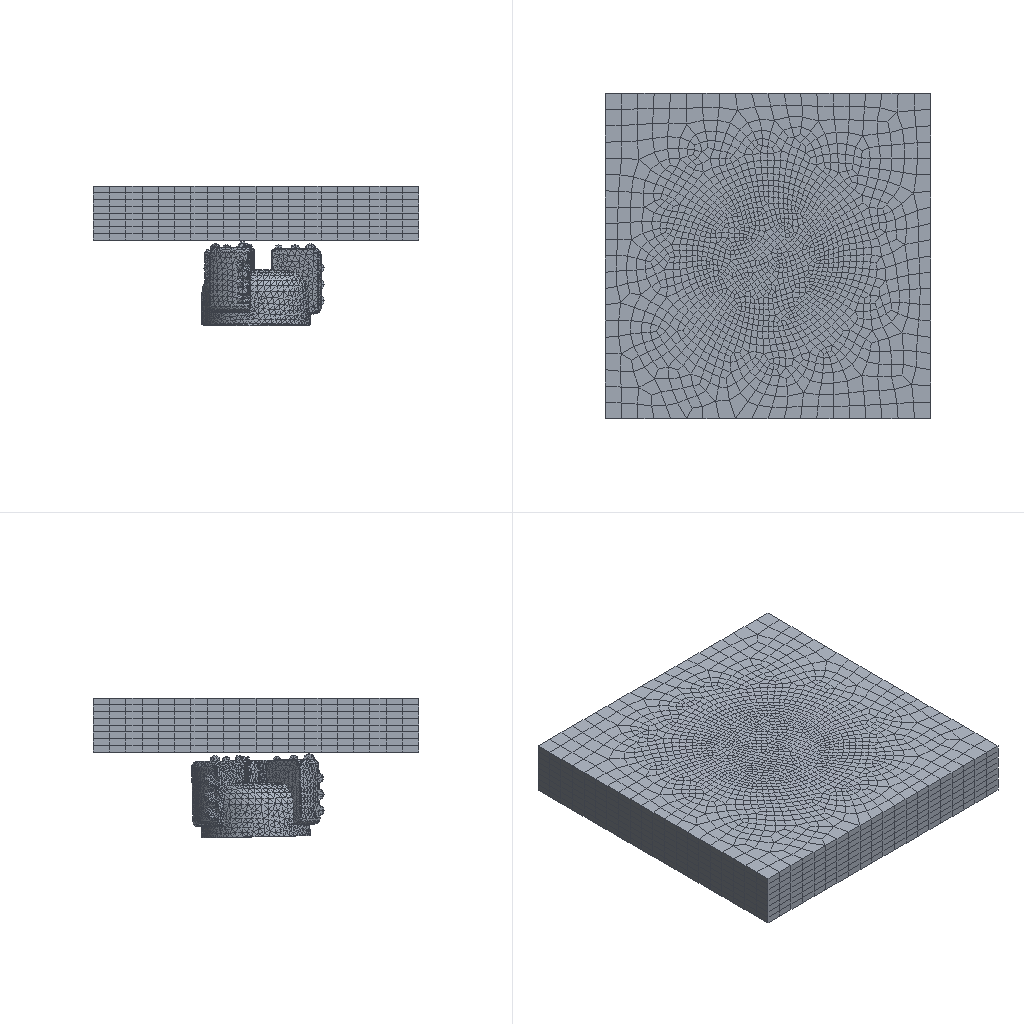Simulation study | abaqus
Set-up summary:
category,name,step,type,value,unit,region
solver,abaqus
solver,version,,,Abaqus/Explicit 2020
units,not stated in the deck,,not stated
analysis,deck,,dynamic temperature-displacement,dynamic temperature-displacement
load_step,Step-1,Step-1,dynamic temperature-displacement,nlgeom=True
contact,interactions,,,general=0 pairs=1 ties=0
load_step,requested,,,1
mesh,nodes,,,23875
mesh,elements,,,46137
element_type,C3D4T,,solid,31481
element_type,C3D8RT,,solid,14656
load,load commands in deck,,count,3
bc,support commands in deck,,count,7
material,SOIL,,in results
material,TOOL,,in results
check,setup vs results,,match,"per instance, exact: element labels, types and connectivity; labels of the nodes the elements use; coordinates of those nodes at SINGLE_PRECISION in 2 of 2 instance(s)"
Abaqus input file, long lists of numbers shortened:
*Heading
** Job name: Job-1 Model name: Model-1
** Generated by: Abaqus/CAE 2020
*Preprint, echo=NO, model=NO, history=NO, contact=NO
**
** PARTS
**
*Part, name=soil
*Node
      1,         300.,        -300.,          50.
      2,         300.,           0.,          50.
** (16855 more lines like these left out)
*Element, type=C3D8RT
   1,   140,   452,   401,   139,  2803,  5010,  4959,  2802
   2,   418,   451,   531,   480,  4976,  5009,  5089,  5038
** (14654 more lines like these left out)
*Nset, nset=Set-1, generate
     1,  16857,      1
*Elset, elset=Set-1, generate
     1,  14656,      1
** Section: work
*Solid Section, elset=Set-1, material=soil
,
*End Part
**
*Part, name=tool
*Node
      1,  -480.298,   391.052,   8285.385
      2,  -485.169,   396.078,   8285.285
** (7016 more lines like these left out)
*Element, type=C3D4T
    1, 3483, 3484, 3485, 3486
    2, 3483, 3487, 3488, 3489
** (31479 more lines like these left out)
*Nset, nset=Set-4, generate
    1,  7018,     1
*Elset, elset=Set-4, generate
     1,  31481,      1
** Section: tool
*Solid Section, elset=Set-4, material=tool
,
*End Part
**
**
** ASSEMBLY
**
*Assembly, name=Assembly
**
*Instance, name=soil-1, part=soil
*End Instance
**
*Instance, name=tool-1, part=tool
  617.913,  -526.596, -8293.248
*End Instance
**
*Node
      1,         150.,        -150.,         -78.
*Nset, nset=Set-1, instance=soil-1
    1,    2,    3,    4,    6,    7,    8,    9,   11,   12,   13,   14,   15,   16,   17,   18
   19,   20,   21,   22,   23,   24,   25,   26,   27,   28,   29,   30,   31,   32,   33,   34
** (43 more lines like these left out)
*Elset, elset=Set-1, instance=soil-1
   26,   41,   55,   68,   69,  745,  763,  765,  770,  775,  783,  817,  825,  833,  837,  838
  842,  847,  854,  855,  859,  866,  868,  869,  876,  877,  881,  882,  888,  892,  894,  903
** (36 more lines like these left out)
*Nset, nset=Set-5
 1,
*Nset, nset=Set-6, instance=soil-1
     5,    10,    87,    88,    89,    90,    91,    92,    93,    94,    95,    96,    97,    98,    99,   100
   101,   102,   103,   104,   105,   106,   107,   108,   109,   110,   111,   112,   113,   114,   115,   116
** (486 more lines like these left out)
*Elset, elset=Set-6, instance=soil-1, generate
  8081,  14656,      1
*Nset, nset=b_Set-3, instance=tool-1, generate
    1,  7018,     1
*Elset, elset=b_Set-3, instance=tool-1, generate
     1,  31481,      1
*Nset, nset=s_Set-2, instance=soil-1
     5,    10,    87,    88,    89,    90,    91,    92,    93,    94,    95,    96,    97,    98,    99,   100
   101,   102,   103,   104,   105,   106,   107,   108,   109,   110,   111,   112,   113,   114,   115,   116
** (486 more lines like these left out)
*Elset, elset=s_Set-2, instance=soil-1, generate
  8081,  14656,      1
*Nset, nset=_PickedSet12, internal
 1,
*Elset, elset=_Surf-2_S2, internal, instance=soil-1, generate
 8081,  8902,     1
*Surface, type=ELEMENT, name=Surf-2
_Surf-2_S2, S2
*Elset, elset=_m_Surf-1_S4, internal, instance=tool-1
   134,   174,   212,   269,   391,   475,   493,   582,   620,   748,   804,   815,   837,   842,   929,   934
   951,   968,   985,   994,  1022,  1129,  1158,  1162,  1171,  1187,  1201,  1401,  1451,  1473,  1483,  1506
** (34 more lines like these left out)
*Elset, elset=_m_Surf-1_S3, internal, instance=tool-1
    48,   141,   145,   213,   218,   230,   242,   255,   258,   354,   387,   439,   484,   532,   563,   573
   750,   886,   891,   895,  1033,  1073,  1080,  1274,  1367,  1379,  1431,  1448,  1510,  1537,  1625,  1787
** (343 more lines like these left out)
*Elset, elset=_m_Surf-1_S2, internal, instance=tool-1
    32,   156,   319,   522,   621,   643,   767,  1266,  1278,  2015,  2118,  2129,  2141,  2446,  2475,  2562
  2711,  2840,  2982,  3113,  3273,  3457,  3683,  4947,  5061,  5123,  5145,  5147,  5207,  5253,  5262,  5294
** (29 more lines like these left out)
*Elset, elset=_m_Surf-1_S1, internal, instance=tool-1
   426,   977,  1090,  1132,  1202,  1289,  1917,  2354,  2826,  3195,  3206,  3211,  3296,  4090,  4267,  4343
  4649,  4851,  5135,  5219,  5299,  5368,  5380,  5481,  5518,  5525,  5530,  5542,  5627,  5650,  5718,  5778
** (24 more lines like these left out)
*Surface, type=ELEMENT, name=m_Surf-1
_m_Surf-1_S4, S4
_m_Surf-1_S3, S3
_m_Surf-1_S2, S2
_m_Surf-1_S1, S1
*Surface, type=NODE, name=s_Set-2_CNS_, internal
s_Set-2, 1.
** Constraint: Constraint-1
*Rigid Body, ref node=_PickedSet12, elset=b_Set-3
*End Assembly
*Amplitude, name=Amp-1, definition=PERIODIC
1,           125.6,              0.,              0.
             1.,              0.
**
** MATERIALS
**
*Material, name=soil
*Conductivity
2.,
*Damage Initiation, criterion=SHEAR
 0.001,0.,0.
*Damage Evolution, type=DISPLACEMENT
 0.0001,
*Density
 2.7e-09,
*Elastic
10500., 0.26
*Plastic
150.,0.
*Specific Heat
 9.6e+08,
*Material, name=tool
*Conductivity
47.,
*Density
 7.7e-09,
*Elastic
210000., 0.3
*Specific Heat
 4.6e+08,
**
** INTERACTION PROPERTIES
**
*Surface Interaction, name=IntProp-1
*Friction
 0.15,
*Surface Behavior, pressure-overclosure=HARD
*Gap Conductance
10000.,  0.
    0., 0.1
** ----------------------------------------------------------------
**
** STEP: Step-1
**
*Step, name=Step-1, nlgeom=YES
*Dynamic Temperature-displacement, Explicit
, 0.5
*Bulk Viscosity
0.06, 1.2
** Mass Scaling: Semi-Automatic
**               Whole Model
*Fixed Mass Scaling, factor=500.
**
** BOUNDARY CONDITIONS
**
** Name: BC-1 Type: 对称/反对称/完全固定
*Boundary
Set-1, ENCASTRE
** Name: [REDACTED] : Speed/Angular velocity
*Boundary, type=VELOCITY
Set-5, 1, 1
Set-5, 2, 2
Set-5, 3, 3, 100.
Set-5, 4, 4
Set-5, 5, 5
Set-5, 6, 6, 31.4
**
** LOADS
**
** Name: Load-2   Type: Body heat flux
*Dflux, amplitude=Amp-1
Set-6, BF, 10000.
**
** INTERACTIONS
**
** Interaction: Int-1
*Contact Pair, interaction=IntProp-1, mechanical constraint=KINEMATIC, cpset=Int-1
m_Surf-1, s_Set-2_CNS_
**
** OUTPUT REQUESTS
**
*Restart, write, number interval=1, time marks=NO
**
** FIELD OUTPUT: F-Output-1
**
*Output, field, number interval=50
*Node Output
A, CF, NT, RF, RFL, RM, RT, U
V
*Element Output, directions=YES
E, EVF, HFL, LE, MISES, MISESMAX, MISESONLY, NE, PE, PEEQ, PEEQMAX, PEEQT, PEEQVAVG, PEMAG, PEVAVG, PRESSONLY
S, SEQUT, SF, SSAVG, STATUS, SVAVG, TEMP, TSHR, YIELDPOT
*Contact Output
CDISP, CFORCE, CSTRESS, CTHICK, FSLIP, FSLIPR, HFLA
**
** HISTORY OUTPUT: H-Output-1
**
*Output, history, variable=PRESELECT
*End Step
Results summary:
result,step,Step-1,completed,increments=18736 time=0.5/0.5
result,analysis,,,"dynamic temperature-displacement, explict"
result,last_loadstep,,,1
result,analysis steps,,count,1
result,primary field,,,"U, NT11"
result,reaction total,,FX,4266.839,model units
result,reaction total,,FY,-5878.168,model units
result,reaction total,,FZ,-22846.891,model units